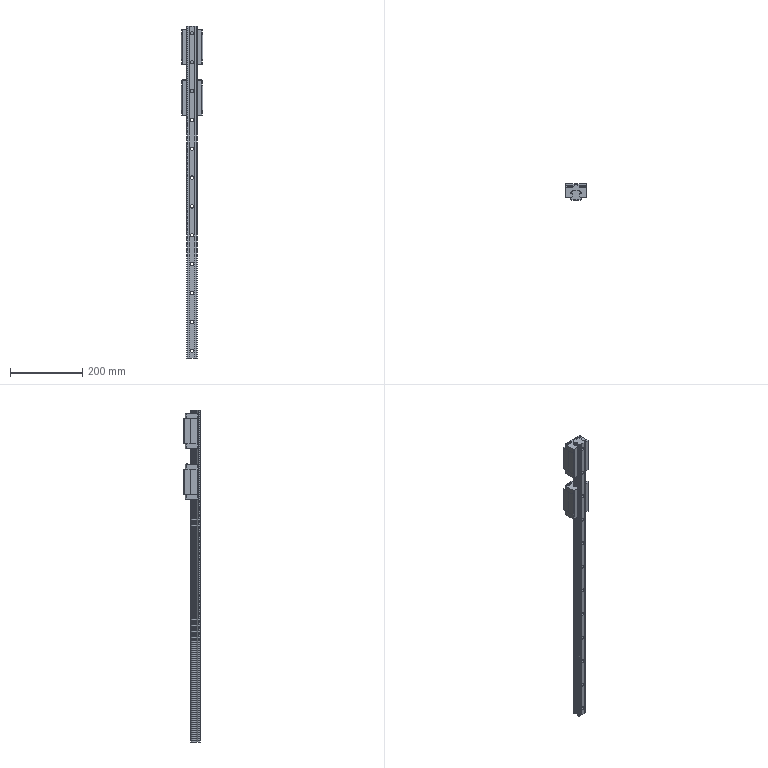Part | SolidWorks | 3 solids | 892 faces | box 60 x 45 x 920 mm | volume 875210 mm3 | plane 646 | cylinder 126 | spline 120 | commonest cylinder face diameters 1.2 x36 9 x24 14 x24 8 x16 1.6 x14 5.66 x12